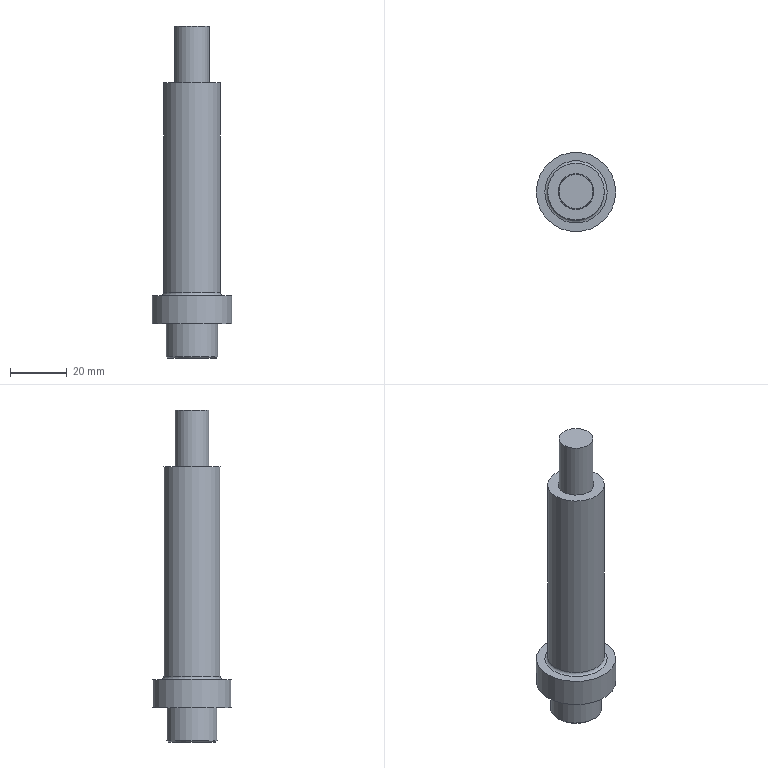Part | STEP file | 1_id630_x_t | 1 solid | 248 faces | box 28 x 28 x 117 mm | volume 33501 mm3 | plane 124 | other 116 | cylinder 5 | cone 2 | torus 1 | commonest cylinder face diameters 12 x1 12.6 x1 18 x1 20 x1 28 x1